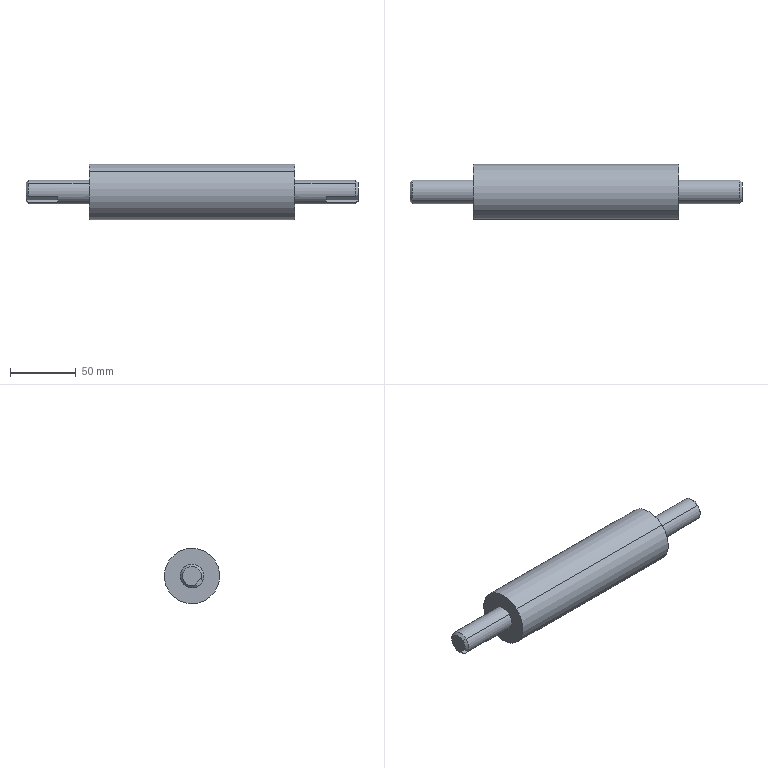Part | NX | 1 solid | 24 faces | box 252 x 42 x 42 mm | volume 239583 mm3 | plane 12 | cone 6 | cylinder 6 | commonest cylinder face diameters 18 x4 42 x2
STEP:
#1=CARTESIAN_POINT('',(256.494,-546.401,2325.36));
#2=VERTEX_POINT('',#1);
#3=CARTESIAN_POINT('',(256.494,-548.336,2317.828));
#4=VERTEX_POINT('',#3);
#5=CARTESIAN_POINT('',(256.494,-541.499,2320.086));
#6=DIRECTION('',(1.,0.,0.));
#7=DIRECTION('',(0.,0.6808,-0.7325));
#8=AXIS2_PLACEMENT_3D('',#5,#6,#7);
#9=CIRCLE('',#8,7.2);
#10=EDGE_CURVE('',#2,#4,#9,.T.);
#11=ORIENTED_EDGE('',*,*,#10,.F.);
#12=CARTESIAN_POINT('',(254.694,-547.626,2326.678));
#13=VERTEX_POINT('',#12);
#14=CARTESIAN_POINT('',(254.694,-547.626,2326.678));
#15=DIRECTION('',(-0.7071,-0.4814,0.5179));
#16=VECTOR('',#15,1.);
#17=LINE('',#14,#16);
#18=EDGE_CURVE('',#2,#13,#17,.T.);
#19=ORIENTED_EDGE('',*,*,#18,.T.);
#20=CARTESIAN_POINT('',(254.694,-549.757,2316.507));
#21=VERTEX_POINT('',#20);
#22=CARTESIAN_POINT('',(254.694,-541.499,2320.086));
#23=DIRECTION('',(-1.,0.,0.));
#24=DIRECTION('',(0.,0.6808,-0.7325));
#25=AXIS2_PLACEMENT_3D('',#22,#23,#24);
#26=CIRCLE('',#25,9.);
#27=EDGE_CURVE('',#21,#13,#26,.T.);
#28=ORIENTED_EDGE('',*,*,#27,.F.);
#29=CARTESIAN_POINT('',(256.494,-548.336,2317.828));
#30=CARTESIAN_POINT('',(255.9,-548.814,2317.383));
#31=CARTESIAN_POINT('',(255.299,-549.287,2316.944));
#32=CARTESIAN_POINT('',(254.694,-549.757,2316.507));
#33=B_SPLINE_CURVE_WITH_KNOTS('',3,(#29,#30,#31,#32),.UNSPECIFIED.,.F.,.F.,(4,4),(0.,1.),.UNSPECIFIED.);
#34=EDGE_CURVE('',#4,#21,#33,.T.);
#35=ORIENTED_EDGE('',*,*,#34,.F.);
#36=EDGE_LOOP('',(#11,#19,#28,#35));
#37=FACE_OUTER_BOUND('',#36,.T.);
#38=CARTESIAN_POINT('',(254.694,-541.499,2320.086));
#39=DIRECTION('',(-1.,0.,0.));
#40=DIRECTION('',(0.,0.6808,-0.7325));
#41=AXIS2_PLACEMENT_3D('',#38,#39,#40);
#42=CONICAL_SURFACE('',#41,9.,45.);
#43=ADVANCED_FACE('',(#37),#42,.T.);
#44=ORIENTED_EDGE('',*,*,#18,.F.);
#45=CARTESIAN_POINT('',(256.494,-536.598,2314.812));
#46=VERTEX_POINT('',#45);
#47=CARTESIAN_POINT('',(256.494,-541.499,2320.086));
#48=DIRECTION('',(1.,0.,0.));
#49=DIRECTION('',(0.,0.6808,-0.7325));
#50=AXIS2_PLACEMENT_3D('',#47,#48,#49);
#51=CIRCLE('',#50,7.2);
#52=EDGE_CURVE('',#46,#2,#51,.T.);
#53=ORIENTED_EDGE('',*,*,#52,.F.);
#54=CARTESIAN_POINT('',(254.694,-535.372,2313.494));
#55=VERTEX_POINT('',#54);
#56=CARTESIAN_POINT('',(254.694,-535.372,2313.494));
#57=DIRECTION('',(-0.7071,0.4814,-0.5179));
#58=VECTOR('',#57,1.);
#59=LINE('',#56,#58);
#60=EDGE_CURVE('',#46,#55,#59,.T.);
#61=ORIENTED_EDGE('',*,*,#60,.T.);
#62=CARTESIAN_POINT('',(254.694,-541.499,2320.086));
#63=DIRECTION('',(-1.,0.,0.));
#64=DIRECTION('',(0.,0.6808,-0.7325));
#65=AXIS2_PLACEMENT_3D('',#62,#63,#64);
#66=CIRCLE('',#65,9.);
#67=EDGE_CURVE('',#13,#55,#66,.T.);
#68=ORIENTED_EDGE('',*,*,#67,.F.);
#69=EDGE_LOOP('',(#44,#53,#61,#68));
#70=FACE_OUTER_BOUND('',#69,.T.);
#71=CARTESIAN_POINT('',(254.694,-541.499,2320.086));
#72=DIRECTION('',(-1.,0.,0.));
#73=DIRECTION('',(0.,0.6808,-0.7325));
#74=AXIS2_PLACEMENT_3D('',#71,#72,#73);
#75=CONICAL_SURFACE('',#74,9.,45.);
#76=ADVANCED_FACE('',(#70),#75,.T.);
#77=ORIENTED_EDGE('',*,*,#27,.T.);
#78=CARTESIAN_POINT('',(208.494,-547.626,2326.678));
#79=VERTEX_POINT('',#78);
#80=CARTESIAN_POINT('',(256.494,-547.626,2326.678));
#81=DIRECTION('',(-1.,0.,0.));
#82=VECTOR('',#81,1.);
#83=LINE('',#80,#82);
#84=EDGE_CURVE('',#13,#79,#83,.T.);
#85=ORIENTED_EDGE('',*,*,#84,.T.);
#86=CARTESIAN_POINT('',(208.494,-535.372,2313.494));
#87=VERTEX_POINT('',#86);
#88=CARTESIAN_POINT('',(208.494,-541.499,2320.086));
#89=DIRECTION('',(-1.,0.,0.));
#90=DIRECTION('',(0.,0.6808,-0.7325));
#91=AXIS2_PLACEMENT_3D('',#88,#89,#90);
#92=CIRCLE('',#91,9.);
#93=EDGE_CURVE('',#87,#79,#92,.T.);
#94=ORIENTED_EDGE('',*,*,#93,.F.);
#95=CARTESIAN_POINT('',(256.494,-535.372,2313.494));
#96=DIRECTION('',(1.,0.,0.));
#97=VECTOR('',#96,1.);
#98=LINE('',#95,#97);
#99=EDGE_CURVE('',#87,#55,#98,.T.);
#100=ORIENTED_EDGE('',*,*,#99,.T.);
#101=CARTESIAN_POINT('',(254.694,-545.672,2312.112));
#102=VERTEX_POINT('',#101);
#103=CARTESIAN_POINT('',(254.694,-541.499,2320.086));
#104=DIRECTION('',(-1.,0.,0.));
#105=DIRECTION('',(0.,0.6808,-0.7325));
#106=AXIS2_PLACEMENT_3D('',#103,#104,#105);
#107=CIRCLE('',#106,9.);
#108=EDGE_CURVE('',#55,#102,#107,.T.);
#109=ORIENTED_EDGE('',*,*,#108,.T.);
#110=CARTESIAN_POINT('',(232.494,-545.672,2312.112));
#111=VERTEX_POINT('',#110);
#112=CARTESIAN_POINT('',(256.494,-545.672,2312.112));
#113=DIRECTION('',(1.,0.,0.));
#114=VECTOR('',#113,1.);
#115=LINE('',#112,#114);
#116=EDGE_CURVE('',#111,#102,#115,.T.);
#117=ORIENTED_EDGE('',*,*,#116,.F.);
#118=CARTESIAN_POINT('',(232.494,-549.757,2316.507));
#119=VERTEX_POINT('',#118);
#120=CARTESIAN_POINT('',(232.494,-541.499,2320.086));
#121=DIRECTION('',(-1.,0.,0.));
#122=DIRECTION('',(0.,-0.6808,0.7325));
#123=AXIS2_PLACEMENT_3D('',#120,#121,#122);
#124=CIRCLE('',#123,9.);
#125=EDGE_CURVE('',#111,#119,#124,.T.);
#126=ORIENTED_EDGE('',*,*,#125,.T.);
#127=CARTESIAN_POINT('',(256.494,-549.757,2316.507));
#128=DIRECTION('',(-1.,0.,0.));
#129=VECTOR('',#128,1.);
#130=LINE('',#127,#129);
#131=EDGE_CURVE('',#21,#119,#130,.T.);
#132=ORIENTED_EDGE('',*,*,#131,.F.);
#133=EDGE_LOOP('',(#77,#85,#94,#100,#109,#117,#126,#132));
#134=FACE_OUTER_BOUND('',#133,.T.);
#135=CARTESIAN_POINT('',(256.494,-541.499,2320.086));
#136=DIRECTION('',(-1.,0.,0.));
#137=DIRECTION('',(0.,0.6808,-0.7325));
#138=AXIS2_PLACEMENT_3D('',#135,#136,#137);
#139=CYLINDRICAL_SURFACE('',#138,9.);
#140=ADVANCED_FACE('',(#134),#139,.T.);
#141=CARTESIAN_POINT('',(208.494,-527.202,2304.704));
#142=VERTEX_POINT('',#141);
#143=CARTESIAN_POINT('',(208.494,-555.796,2335.468));
#144=VERTEX_POINT('',#143);
#145=CARTESIAN_POINT('',(208.494,-541.499,2320.086));
#146=DIRECTION('',(-1.,0.,0.));
#147=DIRECTION('',(0.,0.6808,-0.7325));
#148=AXIS2_PLACEMENT_3D('',#145,#146,#147);
#149=CIRCLE('',#148,21.);
#150=EDGE_CURVE('',#142,#144,#149,.T.);
#151=ORIENTED_EDGE('',*,*,#150,.T.);
#152=CARTESIAN_POINT('',(52.494,-555.796,2335.468));
#153=VERTEX_POINT('',#152);
#154=CARTESIAN_POINT('',(208.494,-555.796,2335.468));
#155=DIRECTION('',(1.,0.,0.));
#156=VECTOR('',#155,1.);
#157=LINE('',#154,#156);
#158=EDGE_CURVE('',#153,#144,#157,.T.);
#159=ORIENTED_EDGE('',*,*,#158,.F.);
#160=CARTESIAN_POINT('',(52.494,-527.202,2304.704));
#161=VERTEX_POINT('',#160);
#162=CARTESIAN_POINT('',(52.494,-541.499,2320.086));
#163=DIRECTION('',(-1.,0.,0.));
#164=DIRECTION('',(0.,0.6808,-0.7325));
#165=AXIS2_PLACEMENT_3D('',#162,#163,#164);
#166=CIRCLE('',#165,21.);
#167=EDGE_CURVE('',#161,#153,#166,.T.);
#168=ORIENTED_EDGE('',*,*,#167,.F.);
#169=CARTESIAN_POINT('',(208.494,-527.202,2304.704));
#170=DIRECTION('',(-1.,0.,0.));
#171=VECTOR('',#170,1.);
#172=LINE('',#169,#171);
#173=EDGE_CURVE('',#142,#161,#172,.T.);
#174=ORIENTED_EDGE('',*,*,#173,.F.);
#175=EDGE_LOOP('',(#151,#159,#168,#174));
#176=FACE_OUTER_BOUND('',#175,.T.);
#177=CARTESIAN_POINT('',(208.494,-541.499,2320.086));
#178=DIRECTION('',(-1.,0.,0.));
#179=DIRECTION('',(0.,0.6808,-0.7325));
#180=AXIS2_PLACEMENT_3D('',#177,#178,#179);
#181=CYLINDRICAL_SURFACE('',#180,21.);
#182=ADVANCED_FACE('',(#176),#181,.T.);
#183=CARTESIAN_POINT('',(4.494,-536.598,2314.812));
#184=VERTEX_POINT('',#183);
#185=CARTESIAN_POINT('',(4.494,-544.251,2313.433));
#186=VERTEX_POINT('',#185);
#187=CARTESIAN_POINT('',(4.494,-541.499,2320.086));
#188=DIRECTION('',(-1.,0.,0.));
#189=DIRECTION('',(0.,0.6808,-0.7325));
#190=AXIS2_PLACEMENT_3D('',#187,#188,#189);
#191=CIRCLE('',#190,7.2);
#192=EDGE_CURVE('',#184,#186,#191,.T.);
#193=ORIENTED_EDGE('',*,*,#192,.F.);
#194=CARTESIAN_POINT('',(6.294,-535.372,2313.494));
#195=VERTEX_POINT('',#194);
#196=CARTESIAN_POINT('',(4.494,-536.598,2314.812));
#197=DIRECTION('',(0.7071,0.4814,-0.5179));
#198=VECTOR('',#197,1.);
#199=LINE('',#196,#198);
#200=EDGE_CURVE('',#184,#195,#199,.T.);
#201=ORIENTED_EDGE('',*,*,#200,.T.);
#202=CARTESIAN_POINT('',(6.294,-545.672,2312.112));
#203=VERTEX_POINT('',#202);
#204=CARTESIAN_POINT('',(6.294,-541.499,2320.086));
#205=DIRECTION('',(1.,0.,0.));
#206=DIRECTION('',(0.,0.6808,-0.7325));
#207=AXIS2_PLACEMENT_3D('',#204,#205,#206);
#208=CIRCLE('',#207,9.);
#209=EDGE_CURVE('',#203,#195,#208,.T.);
#210=ORIENTED_EDGE('',*,*,#209,.F.);
#211=CARTESIAN_POINT('',(6.294,-545.672,2312.112));
#212=CARTESIAN_POINT('',(5.688,-545.202,2312.549));
#213=CARTESIAN_POINT('',(5.087,-544.729,2312.988));
#214=CARTESIAN_POINT('',(4.494,-544.251,2313.433));
#215=B_SPLINE_CURVE_WITH_KNOTS('',3,(#211,#212,#213,#214),.UNSPECIFIED.,.F.,.F.,(4,4),(0.,1.),.UNSPECIFIED.);
#216=EDGE_CURVE('',#203,#186,#215,.T.);
#217=ORIENTED_EDGE('',*,*,#216,.T.);
#218=EDGE_LOOP('',(#193,#201,#210,#217));
#219=FACE_OUTER_BOUND('',#218,.T.);
#220=CARTESIAN_POINT('',(4.494,-541.499,2320.086));
#221=DIRECTION('',(1.,0.,0.));
#222=DIRECTION('',(0.,-0.6808,0.7325));
#223=AXIS2_PLACEMENT_3D('',#220,#221,#222);
#224=CONICAL_SURFACE('',#223,7.2,45.);
#225=ADVANCED_FACE('',(#219),#224,.T.);
#226=ORIENTED_EDGE('',*,*,#200,.F.);
#227=CARTESIAN_POINT('',(4.494,-546.401,2325.36));
#228=VERTEX_POINT('',#227);
#229=CARTESIAN_POINT('',(4.494,-541.499,2320.086));
#230=DIRECTION('',(-1.,0.,0.));
#231=DIRECTION('',(0.,0.6808,-0.7325));
#232=AXIS2_PLACEMENT_3D('',#229,#230,#231);
#233=CIRCLE('',#232,7.2);
#234=EDGE_CURVE('',#228,#184,#233,.T.);
#235=ORIENTED_EDGE('',*,*,#234,.F.);
#236=CARTESIAN_POINT('',(6.294,-547.626,2326.678));
#237=VERTEX_POINT('',#236);
#238=CARTESIAN_POINT('',(4.494,-546.401,2325.36));
#239=DIRECTION('',(0.7071,-0.4814,0.5179));
#240=VECTOR('',#239,1.);
#241=LINE('',#238,#240);
#242=EDGE_CURVE('',#228,#237,#241,.T.);
#243=ORIENTED_EDGE('',*,*,#242,.T.);
#244=CARTESIAN_POINT('',(6.294,-541.499,2320.086));
#245=DIRECTION('',(1.,0.,0.));
#246=DIRECTION('',(0.,0.6808,-0.7325));
#247=AXIS2_PLACEMENT_3D('',#244,#245,#246);
#248=CIRCLE('',#247,9.);
#249=EDGE_CURVE('',#195,#237,#248,.T.);
#250=ORIENTED_EDGE('',*,*,#249,.F.);
#251=EDGE_LOOP('',(#226,#235,#243,#250));
#252=FACE_OUTER_BOUND('',#251,.T.);
#253=CARTESIAN_POINT('',(4.494,-541.499,2320.086));
#254=DIRECTION('',(1.,0.,0.));
#255=DIRECTION('',(0.,-0.6808,0.7325));
#256=AXIS2_PLACEMENT_3D('',#253,#254,#255);
#257=CONICAL_SURFACE('',#256,7.2,45.);
#258=ADVANCED_FACE('',(#252),#257,.T.);
#259=CARTESIAN_POINT('',(52.494,-535.372,2313.494));
#260=VERTEX_POINT('',#259);
#261=CARTESIAN_POINT('',(52.494,-547.626,2326.678));
#262=VERTEX_POINT('',#261);
#263=CARTESIAN_POINT('',(52.494,-541.499,2320.086));
#264=DIRECTION('',(-1.,0.,0.));
#265=DIRECTION('',(0.,0.6808,-0.7325));
#266=AXIS2_PLACEMENT_3D('',#263,#264,#265);
#267=CIRCLE('',#266,9.);
#268=EDGE_CURVE('',#260,#262,#267,.T.);
#269=ORIENTED_EDGE('',*,*,#268,.T.);
#270=CARTESIAN_POINT('',(256.494,-547.626,2326.678));
#271=DIRECTION('',(1.,0.,0.));
#272=VECTOR('',#271,1.);
#273=LINE('',#270,#272);
#274=EDGE_CURVE('',#237,#262,#273,.T.);
#275=ORIENTED_EDGE('',*,*,#274,.F.);
#276=CARTESIAN_POINT('',(6.294,-549.757,2316.507));
#277=VERTEX_POINT('',#276);
#278=CARTESIAN_POINT('',(6.294,-541.499,2320.086));
#279=DIRECTION('',(1.,0.,0.));
#280=DIRECTION('',(0.,0.6808,-0.7325));
#281=AXIS2_PLACEMENT_3D('',#278,#279,#280);
#282=CIRCLE('',#281,9.);
#283=EDGE_CURVE('',#237,#277,#282,.T.);
#284=ORIENTED_EDGE('',*,*,#283,.T.);
#285=CARTESIAN_POINT('',(28.494,-549.757,2316.507));
#286=VERTEX_POINT('',#285);
#287=CARTESIAN_POINT('',(256.494,-549.757,2316.507));
#288=DIRECTION('',(1.,0.,0.));
#289=VECTOR('',#288,1.);
#290=LINE('',#287,#289);
#291=EDGE_CURVE('',#277,#286,#290,.T.);
#292=ORIENTED_EDGE('',*,*,#291,.T.);
#293=CARTESIAN_POINT('',(28.494,-545.672,2312.112));
#294=VERTEX_POINT('',#293);
#295=CARTESIAN_POINT('',(28.494,-541.499,2320.086));
#296=DIRECTION('',(1.,0.,0.));
#297=DIRECTION('',(0.,0.6808,-0.7325));
#298=AXIS2_PLACEMENT_3D('',#295,#296,#297);
#299=CIRCLE('',#298,9.);
#300=EDGE_CURVE('',#286,#294,#299,.T.);
#301=ORIENTED_EDGE('',*,*,#300,.T.);
#302=CARTESIAN_POINT('',(256.494,-545.672,2312.112));
#303=DIRECTION('',(-1.,0.,0.));
#304=VECTOR('',#303,1.);
#305=LINE('',#302,#304);
#306=EDGE_CURVE('',#294,#203,#305,.T.);
#307=ORIENTED_EDGE('',*,*,#306,.T.);
#308=ORIENTED_EDGE('',*,*,#209,.T.);
#309=CARTESIAN_POINT('',(256.494,-535.372,2313.494));
#310=DIRECTION('',(-1.,0.,0.));
#311=VECTOR('',#310,1.);
#312=LINE('',#309,#311);
#313=EDGE_CURVE('',#260,#195,#312,.T.);
#314=ORIENTED_EDGE('',*,*,#313,.F.);
#315=EDGE_LOOP('',(#269,#275,#284,#292,#301,#307,#308,#314));
#316=FACE_OUTER_BOUND('',#315,.T.);
#317=CARTESIAN_POINT('',(256.494,-541.499,2320.086));
#318=DIRECTION('',(-1.,0.,0.));
#319=DIRECTION('',(0.,0.6808,-0.7325));
#320=AXIS2_PLACEMENT_3D('',#317,#318,#319);
#321=CYLINDRICAL_SURFACE('',#320,9.);
#322=ADVANCED_FACE('',(#316),#321,.T.);
#323=CARTESIAN_POINT('',(4.494,-548.336,2317.828));
#324=VERTEX_POINT('',#323);
#325=CARTESIAN_POINT('',(4.494,-541.499,2320.086));
#326=DIRECTION('',(-1.,0.,0.));
#327=DIRECTION('',(0.,0.6808,-0.7325));
#328=AXIS2_PLACEMENT_3D('',#325,#326,#327);
#329=CIRCLE('',#328,7.2);
#330=EDGE_CURVE('',#324,#228,#329,.T.);
#331=ORIENTED_EDGE('',*,*,#330,.T.);
#332=ORIENTED_EDGE('',*,*,#234,.T.);
#333=ORIENTED_EDGE('',*,*,#192,.T.);
#334=CARTESIAN_POINT('',(4.494,-543.852,2313.804));
#335=VERTEX_POINT('',#334);
#336=CARTESIAN_POINT('',(4.494,-549.565,2308.494));
#337=DIRECTION('',(0.,0.7325,0.6808));
#338=VECTOR('',#337,1.);
#339=LINE('',#336,#338);
#340=EDGE_CURVE('',#186,#335,#339,.T.);
#341=ORIENTED_EDGE('',*,*,#340,.T.);
#342=CARTESIAN_POINT('',(4.494,-547.936,2318.199));
#343=VERTEX_POINT('',#342);
#344=CARTESIAN_POINT('',(4.494,-543.852,2313.804));
#345=DIRECTION('',(0.,-0.6808,0.7325));
#346=VECTOR('',#345,1.);
#347=LINE('',#344,#346);
#348=EDGE_CURVE('',#335,#343,#347,.T.);
#349=ORIENTED_EDGE('',*,*,#348,.T.);
#350=CARTESIAN_POINT('',(4.494,-553.65,2312.889));
#351=DIRECTION('',(0.,-0.7325,-0.6808));
#352=VECTOR('',#351,1.);
#353=LINE('',#350,#352);
#354=EDGE_CURVE('',#343,#324,#353,.T.);
#355=ORIENTED_EDGE('',*,*,#354,.T.);
#356=EDGE_LOOP('',(#331,#332,#333,#341,#349,#355));
#357=FACE_OUTER_BOUND('',#356,.T.);
#358=CARTESIAN_POINT('',(4.494,-541.499,2320.086));
#359=DIRECTION('',(-1.,0.,0.));
#360=DIRECTION('',(0.,0.6808,-0.7325));
#361=AXIS2_PLACEMENT_3D('',#358,#359,#360);
#362=PLANE('',#361);
#363=ADVANCED_FACE('',(#357),#362,.T.);
#364=ORIENTED_EDGE('',*,*,#274,.T.);
#365=CARTESIAN_POINT('',(52.494,-541.499,2320.086));
#366=DIRECTION('',(-1.,0.,0.));
#367=DIRECTION('',(0.,0.6808,-0.7325));
#368=AXIS2_PLACEMENT_3D('',#365,#366,#367);
#369=CIRCLE('',#368,9.);
#370=EDGE_CURVE('',#262,#260,#369,.T.);
#371=ORIENTED_EDGE('',*,*,#370,.T.);
#372=ORIENTED_EDGE('',*,*,#313,.T.);
#373=ORIENTED_EDGE('',*,*,#249,.T.);
#374=EDGE_LOOP('',(#364,#371,#372,#373));
#375=FACE_OUTER_BOUND('',#374,.T.);
#376=CARTESIAN_POINT('',(256.494,-541.499,2320.086));
#377=DIRECTION('',(-1.,0.,0.));
#378=DIRECTION('',(0.,0.6808,-0.7325));
#379=AXIS2_PLACEMENT_3D('',#376,#377,#378);
#380=CYLINDRICAL_SURFACE('',#379,9.);
#381=ADVANCED_FACE('',(#375),#380,.T.);
#382=ORIENTED_EDGE('',*,*,#242,.F.);
#383=ORIENTED_EDGE('',*,*,#330,.F.);
#384=CARTESIAN_POINT('',(4.494,-548.336,2317.828));
#385=CARTESIAN_POINT('',(5.087,-548.814,2317.383));
#386=CARTESIAN_POINT('',(5.688,-549.287,2316.944));
#387=CARTESIAN_POINT('',(6.294,-549.757,2316.507));
#388=B_SPLINE_CURVE_WITH_KNOTS('',3,(#384,#385,#386,#387),.UNSPECIFIED.,.F.,.F.,(4,4),(0.,1.),.UNSPECIFIED.);
#389=EDGE_CURVE('',#324,#277,#388,.T.);
#390=ORIENTED_EDGE('',*,*,#389,.T.);
#391=ORIENTED_EDGE('',*,*,#283,.F.);
#392=EDGE_LOOP('',(#382,#383,#390,#391));
#393=FACE_OUTER_BOUND('',#392,.T.);
#394=CARTESIAN_POINT('',(4.494,-541.499,2320.086));
#395=DIRECTION('',(1.,0.,0.));
#396=DIRECTION('',(0.,-0.6808,0.7325));
#397=AXIS2_PLACEMENT_3D('',#394,#395,#396);
#398=CONICAL_SURFACE('',#397,7.2,45.);
#399=ADVANCED_FACE('',(#393),#398,.T.);
#400=ORIENTED_EDGE('',*,*,#158,.T.);
#401=CARTESIAN_POINT('',(208.494,-541.499,2320.086));
#402=DIRECTION('',(-1.,0.,0.));
#403=DIRECTION('',(0.,0.6808,-0.7325));
#404=AXIS2_PLACEMENT_3D('',#401,#402,#403);
#405=CIRCLE('',#404,21.);
#406=EDGE_CURVE('',#144,#142,#405,.T.);
#407=ORIENTED_EDGE('',*,*,#406,.T.);
#408=ORIENTED_EDGE('',*,*,#173,.T.);
#409=CARTESIAN_POINT('',(52.494,-541.499,2320.086));
#410=DIRECTION('',(-1.,0.,0.));
#411=DIRECTION('',(0.,0.6808,-0.7325));
#412=AXIS2_PLACEMENT_3D('',#409,#410,#411);
#413=CIRCLE('',#412,21.);
#414=EDGE_CURVE('',#153,#161,#413,.T.);
#415=ORIENTED_EDGE('',*,*,#414,.F.);
#416=EDGE_LOOP('',(#400,#407,#408,#415));
#417=FACE_OUTER_BOUND('',#416,.T.);
#418=CARTESIAN_POINT('',(208.494,-541.499,2320.086));
#419=DIRECTION('',(-1.,0.,0.));
#420=DIRECTION('',(0.,0.6808,-0.7325));
#421=AXIS2_PLACEMENT_3D('',#418,#419,#420);
#422=CYLINDRICAL_SURFACE('',#421,21.);
#423=ADVANCED_FACE('',(#417),#422,.T.);
#424=ORIENTED_EDGE('',*,*,#93,.T.);
#425=CARTESIAN_POINT('',(208.494,-541.499,2320.086));
#426=DIRECTION('',(-1.,0.,0.));
#427=DIRECTION('',(0.,0.6808,-0.7325));
#428=AXIS2_PLACEMENT_3D('',#425,#426,#427);
#429=CIRCLE('',#428,9.);
#430=EDGE_CURVE('',#79,#87,#429,.T.);
#431=ORIENTED_EDGE('',*,*,#430,.T.);
#432=EDGE_LOOP('',(#424,#431));
#433=FACE_BOUND('',#432,.T.);
#434=ORIENTED_EDGE('',*,*,#150,.F.);
#435=ORIENTED_EDGE('',*,*,#406,.F.);
#436=EDGE_LOOP('',(#434,#435));
#437=FACE_BOUND('',#436,.T.);
#438=CARTESIAN_POINT('',(208.494,-541.499,2320.086));
#439=DIRECTION('',(-1.,0.,0.));
#440=DIRECTION('',(0.,0.6808,-0.7325));
#441=AXIS2_PLACEMENT_3D('',#438,#439,#440);
#442=PLANE('',#441);
#443=ADVANCED_FACE('',(#433,#437),#442,.F.);
#444=ORIENTED_EDGE('',*,*,#268,.F.);
#445=ORIENTED_EDGE('',*,*,#370,.F.);
#446=EDGE_LOOP('',(#444,#445));
#447=FACE_BOUND('',#446,.T.);
#448=ORIENTED_EDGE('',*,*,#167,.T.);
#449=ORIENTED_EDGE('',*,*,#414,.T.);
#450=EDGE_LOOP('',(#448,#449));
#451=FACE_BOUND('',#450,.T.);
#452=CARTESIAN_POINT('',(52.494,-541.499,2320.086));
#453=DIRECTION('',(-1.,0.,0.));
#454=DIRECTION('',(0.,0.6808,-0.7325));
#455=AXIS2_PLACEMENT_3D('',#452,#453,#454);
#456=PLANE('',#455);
#457=ADVANCED_FACE('',(#447,#451),#456,.T.);
#458=ORIENTED_EDGE('',*,*,#84,.F.);
#459=ORIENTED_EDGE('',*,*,#67,.T.);
#460=ORIENTED_EDGE('',*,*,#99,.F.);
#461=ORIENTED_EDGE('',*,*,#430,.F.);
#462=EDGE_LOOP('',(#458,#459,#460,#461));
#463=FACE_OUTER_BOUND('',#462,.T.);
#464=CARTESIAN_POINT('',(256.494,-541.499,2320.086));
#465=DIRECTION('',(-1.,0.,0.));
#466=DIRECTION('',(0.,0.6808,-0.7325));
#467=AXIS2_PLACEMENT_3D('',#464,#465,#466);
#468=CYLINDRICAL_SURFACE('',#467,9.);
#469=ADVANCED_FACE('',(#463),#468,.T.);
#470=CARTESIAN_POINT('',(256.494,-543.852,2313.804));
#471=VERTEX_POINT('',#470);
#472=CARTESIAN_POINT('',(256.494,-547.936,2318.199));
#473=VERTEX_POINT('',#472);
#474=CARTESIAN_POINT('',(256.494,-543.852,2313.804));
#475=DIRECTION('',(0.,-0.6808,0.7325));
#476=VECTOR('',#475,1.);
#477=LINE('',#474,#476);
#478=EDGE_CURVE('',#471,#473,#477,.T.);
#479=ORIENTED_EDGE('',*,*,#478,.F.);
#480=CARTESIAN_POINT('',(256.494,-544.251,2313.433));
#481=VERTEX_POINT('',#480);
#482=CARTESIAN_POINT('',(256.494,-549.565,2308.494));
#483=DIRECTION('',(0.,0.7325,0.6808));
#484=VECTOR('',#483,1.);
#485=LINE('',#482,#484);
#486=EDGE_CURVE('',#481,#471,#485,.T.);
#487=ORIENTED_EDGE('',*,*,#486,.F.);
#488=CARTESIAN_POINT('',(256.494,-541.499,2320.086));
#489=DIRECTION('',(1.,0.,0.));
#490=DIRECTION('',(0.,0.6808,-0.7325));
#491=AXIS2_PLACEMENT_3D('',#488,#489,#490);
#492=CIRCLE('',#491,7.2);
#493=EDGE_CURVE('',#481,#46,#492,.T.);
#494=ORIENTED_EDGE('',*,*,#493,.T.);
#495=ORIENTED_EDGE('',*,*,#52,.T.);
#496=ORIENTED_EDGE('',*,*,#10,.T.);
#497=CARTESIAN_POINT('',(256.494,-553.65,2312.889));
#498=DIRECTION('',(0.,-0.7325,-0.6808));
#499=VECTOR('',#498,1.);
#500=LINE('',#497,#499);
#501=EDGE_CURVE('',#473,#4,#500,.T.);
#502=ORIENTED_EDGE('',*,*,#501,.F.);
#503=EDGE_LOOP('',(#479,#487,#494,#495,#496,#502));
#504=FACE_OUTER_BOUND('',#503,.T.);
#505=CARTESIAN_POINT('',(256.494,-541.499,2320.086));
#506=DIRECTION('',(-1.,0.,0.));
#507=DIRECTION('',(0.,0.6808,-0.7325));
#508=AXIS2_PLACEMENT_3D('',#505,#506,#507);
#509=PLANE('',#508);
#510=ADVANCED_FACE('',(#504),#509,.F.);
#511=ORIENTED_EDGE('',*,*,#60,.F.);
#512=ORIENTED_EDGE('',*,*,#493,.F.);
#513=CARTESIAN_POINT('',(254.694,-545.672,2312.112));
#514=CARTESIAN_POINT('',(255.299,-545.202,2312.549));
#515=CARTESIAN_POINT('',(255.9,-544.729,2312.988));
#516=CARTESIAN_POINT('',(256.494,-544.251,2313.433));
#517=B_SPLINE_CURVE_WITH_KNOTS('',3,(#513,#514,#515,#516),.UNSPECIFIED.,.F.,.F.,(4,4),(0.,1.),.UNSPECIFIED.);
#518=EDGE_CURVE('',#102,#481,#517,.T.);
#519=ORIENTED_EDGE('',*,*,#518,.F.);
#520=ORIENTED_EDGE('',*,*,#108,.F.);
#521=EDGE_LOOP('',(#511,#512,#519,#520));
#522=FACE_OUTER_BOUND('',#521,.T.);
#523=CARTESIAN_POINT('',(254.694,-541.499,2320.086));
#524=DIRECTION('',(-1.,0.,0.));
#525=DIRECTION('',(0.,0.6808,-0.7325));
#526=AXIS2_PLACEMENT_3D('',#523,#524,#525);
#527=CONICAL_SURFACE('',#526,9.,45.);
#528=ADVANCED_FACE('',(#522),#527,.T.);
#529=ORIENTED_EDGE('',*,*,#116,.T.);
#530=ORIENTED_EDGE('',*,*,#518,.T.);
#531=ORIENTED_EDGE('',*,*,#486,.T.);
#532=CARTESIAN_POINT('',(232.494,-543.852,2313.804));
#533=VERTEX_POINT('',#532);
#534=CARTESIAN_POINT('',(232.494,-543.852,2313.804));
#535=DIRECTION('',(1.,0.,0.));
#536=VECTOR('',#535,1.);
#537=LINE('',#534,#536);
#538=EDGE_CURVE('',#533,#471,#537,.T.);
#539=ORIENTED_EDGE('',*,*,#538,.F.);
#540=CARTESIAN_POINT('',(232.494,-549.565,2308.494));
#541=DIRECTION('',(0.,0.7325,0.6808));
#542=VECTOR('',#541,1.);
#543=LINE('',#540,#542);
#544=EDGE_CURVE('',#111,#533,#543,.T.);
#545=ORIENTED_EDGE('',*,*,#544,.F.);
#546=EDGE_LOOP('',(#529,#530,#531,#539,#545));
#547=FACE_OUTER_BOUND('',#546,.T.);
#548=CARTESIAN_POINT('',(232.494,-549.565,2308.494));
#549=DIRECTION('',(0.,0.6808,-0.7325));
#550=DIRECTION('',(0.,-0.7325,-0.6808));
#551=AXIS2_PLACEMENT_3D('',#548,#549,#550);
#552=PLANE('',#551);
#553=ADVANCED_FACE('',(#547),#552,.F.);
#554=ORIENTED_EDGE('',*,*,#131,.T.);
#555=CARTESIAN_POINT('',(232.494,-547.936,2318.199));
#556=VERTEX_POINT('',#555);
#557=CARTESIAN_POINT('',(232.494,-553.65,2312.889));
#558=DIRECTION('',(0.,-0.7325,-0.6808));
#559=VECTOR('',#558,1.);
#560=LINE('',#557,#559);
#561=EDGE_CURVE('',#556,#119,#560,.T.);
#562=ORIENTED_EDGE('',*,*,#561,.F.);
#563=CARTESIAN_POINT('',(232.494,-547.936,2318.199));
#564=DIRECTION('',(1.,0.,0.));
#565=VECTOR('',#564,1.);
#566=LINE('',#563,#565);
#567=EDGE_CURVE('',#556,#473,#566,.T.);
#568=ORIENTED_EDGE('',*,*,#567,.T.);
#569=ORIENTED_EDGE('',*,*,#501,.T.);
#570=ORIENTED_EDGE('',*,*,#34,.T.);
#571=EDGE_LOOP('',(#554,#562,#568,#569,#570));
#572=FACE_OUTER_BOUND('',#571,.T.);
#573=CARTESIAN_POINT('',(232.494,-553.65,2312.889));
#574=DIRECTION('',(0.,-0.6808,0.7325));
#575=DIRECTION('',(0.,0.7325,0.6808));
#576=AXIS2_PLACEMENT_3D('',#573,#574,#575);
#577=PLANE('',#576);
#578=ADVANCED_FACE('',(#572),#577,.F.);
#579=ORIENTED_EDGE('',*,*,#478,.T.);
#580=ORIENTED_EDGE('',*,*,#567,.F.);
#581=CARTESIAN_POINT('',(232.494,-543.852,2313.804));
#582=DIRECTION('',(0.,-0.6808,0.7325));
#583=VECTOR('',#582,1.);
#584=LINE('',#581,#583);
#585=EDGE_CURVE('',#533,#556,#584,.T.);
#586=ORIENTED_EDGE('',*,*,#585,.F.);
#587=ORIENTED_EDGE('',*,*,#538,.T.);
#588=EDGE_LOOP('',(#579,#580,#586,#587));
#589=FACE_OUTER_BOUND('',#588,.T.);
#590=CARTESIAN_POINT('',(232.494,-543.852,2313.804));
#591=DIRECTION('',(0.,0.7325,0.6808));
#592=DIRECTION('',(0.,0.6808,-0.7325));
#593=AXIS2_PLACEMENT_3D('',#590,#591,#592);
#594=PLANE('',#593);
#595=ADVANCED_FACE('',(#589),#594,.F.);
#596=ORIENTED_EDGE('',*,*,#544,.T.);
#597=ORIENTED_EDGE('',*,*,#585,.T.);
#598=ORIENTED_EDGE('',*,*,#561,.T.);
#599=ORIENTED_EDGE('',*,*,#125,.F.);
#600=EDGE_LOOP('',(#596,#597,#598,#599));
#601=FACE_OUTER_BOUND('',#600,.T.);
#602=CARTESIAN_POINT('',(232.494,-543.852,2313.804));
#603=DIRECTION('',(1.,0.,0.));
#604=DIRECTION('',(0.,-0.6808,0.7325));
#605=AXIS2_PLACEMENT_3D('',#602,#603,#604);
#606=PLANE('',#605);
#607=ADVANCED_FACE('',(#601),#606,.T.);
#608=CARTESIAN_POINT('',(28.494,-543.852,2313.804));
#609=VERTEX_POINT('',#608);
#610=CARTESIAN_POINT('',(28.494,-549.565,2308.494));
#611=DIRECTION('',(0.,0.7325,0.6808));
#612=VECTOR('',#611,1.);
#613=LINE('',#610,#612);
#614=EDGE_CURVE('',#294,#609,#613,.T.);
#615=ORIENTED_EDGE('',*,*,#614,.T.);
#616=CARTESIAN_POINT('',(28.494,-543.852,2313.804));
#617=DIRECTION('',(-1.,0.,0.));
#618=VECTOR('',#617,1.);
#619=LINE('',#616,#618);
#620=EDGE_CURVE('',#609,#335,#619,.T.);
#621=ORIENTED_EDGE('',*,*,#620,.T.);
#622=ORIENTED_EDGE('',*,*,#340,.F.);
#623=ORIENTED_EDGE('',*,*,#216,.F.);
#624=ORIENTED_EDGE('',*,*,#306,.F.);
#625=EDGE_LOOP('',(#615,#621,#622,#623,#624));
#626=FACE_OUTER_BOUND('',#625,.T.);
#627=CARTESIAN_POINT('',(28.494,-549.565,2308.494));
#628=DIRECTION('',(0.,-0.6808,0.7325));
#629=DIRECTION('',(0.,0.7325,0.6808));
#630=AXIS2_PLACEMENT_3D('',#627,#628,#629);
#631=PLANE('',#630);
#632=ADVANCED_FACE('',(#626),#631,.T.);
#633=ORIENTED_EDGE('',*,*,#348,.F.);
#634=ORIENTED_EDGE('',*,*,#620,.F.);
#635=CARTESIAN_POINT('',(28.494,-547.936,2318.199));
#636=VERTEX_POINT('',#635);
#637=CARTESIAN_POINT('',(28.494,-543.852,2313.804));
#638=DIRECTION('',(0.,-0.6808,0.7325));
#639=VECTOR('',#638,1.);
#640=LINE('',#637,#639);
#641=EDGE_CURVE('',#609,#636,#640,.T.);
#642=ORIENTED_EDGE('',*,*,#641,.T.);
#643=CARTESIAN_POINT('',(28.494,-547.936,2318.199));
#644=DIRECTION('',(-1.,0.,0.));
#645=VECTOR('',#644,1.);
#646=LINE('',#643,#645);
#647=EDGE_CURVE('',#636,#343,#646,.T.);
#648=ORIENTED_EDGE('',*,*,#647,.T.);
#649=EDGE_LOOP('',(#633,#634,#642,#648));
#650=FACE_OUTER_BOUND('',#649,.T.);
#651=CARTESIAN_POINT('',(28.494,-543.852,2313.804));
#652=DIRECTION('',(0.,-0.7325,-0.6808));
#653=DIRECTION('',(0.,-0.6808,0.7325));
#654=AXIS2_PLACEMENT_3D('',#651,#652,#653);
#655=PLANE('',#654);
#656=ADVANCED_FACE('',(#650),#655,.T.);
#657=ORIENTED_EDGE('',*,*,#389,.F.);
#658=ORIENTED_EDGE('',*,*,#354,.F.);
#659=ORIENTED_EDGE('',*,*,#647,.F.);
#660=CARTESIAN_POINT('',(28.494,-553.65,2312.889));
#661=DIRECTION('',(0.,-0.7325,-0.6808));
#662=VECTOR('',#661,1.);
#663=LINE('',#660,#662);
#664=EDGE_CURVE('',#636,#286,#663,.T.);
#665=ORIENTED_EDGE('',*,*,#664,.T.);
#666=ORIENTED_EDGE('',*,*,#291,.F.);
#667=EDGE_LOOP('',(#657,#658,#659,#665,#666));
#668=FACE_OUTER_BOUND('',#667,.T.);
#669=CARTESIAN_POINT('',(28.494,-553.65,2312.889));
#670=DIRECTION('',(0.,0.6808,-0.7325));
#671=DIRECTION('',(0.,-0.7325,-0.6808));
#672=AXIS2_PLACEMENT_3D('',#669,#670,#671);
#673=PLANE('',#672);
#674=ADVANCED_FACE('',(#668),#673,.T.);
#675=ORIENTED_EDGE('',*,*,#664,.F.);
#676=ORIENTED_EDGE('',*,*,#641,.F.);
#677=ORIENTED_EDGE('',*,*,#614,.F.);
#678=ORIENTED_EDGE('',*,*,#300,.F.);
#679=EDGE_LOOP('',(#675,#676,#677,#678));
#680=FACE_OUTER_BOUND('',#679,.T.);
#681=CARTESIAN_POINT('',(28.494,-543.852,2313.804));
#682=DIRECTION('',(-1.,0.,0.));
#683=DIRECTION('',(0.,-0.6808,0.7325));
#684=AXIS2_PLACEMENT_3D('',#681,#682,#683);
#685=PLANE('',#684);
#686=ADVANCED_FACE('',(#680),#685,.T.);
#687=CLOSED_SHELL('',(#43,#76,#140,#182,#225,#258,#322,#363,#381,#399,#423,#443,#457,#469,#510,#528,#553,#578,#595,#607,#632,#656,#674,#686));
#688=MANIFOLD_SOLID_BREP('',#687);
#689=(LENGTH_UNIT()NAMED_UNIT(*)SI_UNIT(.MILLI.,.METRE.));
#690=UNCERTAINTY_MEASURE_WITH_UNIT(LENGTH_MEASURE(0.0508),#689,'','');
#691=(NAMED_UNIT(*)PLANE_ANGLE_UNIT()SI_UNIT($,.RADIAN.));
#692=PLANE_ANGLE_MEASURE_WITH_UNIT(PLANE_ANGLE_MEASURE(0.01745),#691);
#693=DIMENSIONAL_EXPONENTS(0.,0.,0.,0.,0.,0.,0.);
#694=(CONVERSION_BASED_UNIT('DEGREE',#692)NAMED_UNIT(#693)PLANE_ANGLE_UNIT());
#695=(NAMED_UNIT(*)SI_UNIT($,.STERADIAN.)SOLID_ANGLE_UNIT());
#696=(GEOMETRIC_REPRESENTATION_CONTEXT(3)GLOBAL_UNCERTAINTY_ASSIGNED_CONTEXT((#690))GLOBAL_UNIT_ASSIGNED_CONTEXT((#689,#694,#695))REPRESENTATION_CONTEXT('',''));
#697=ADVANCED_BREP_SHAPE_REPRESENTATION('',(#688),#696);